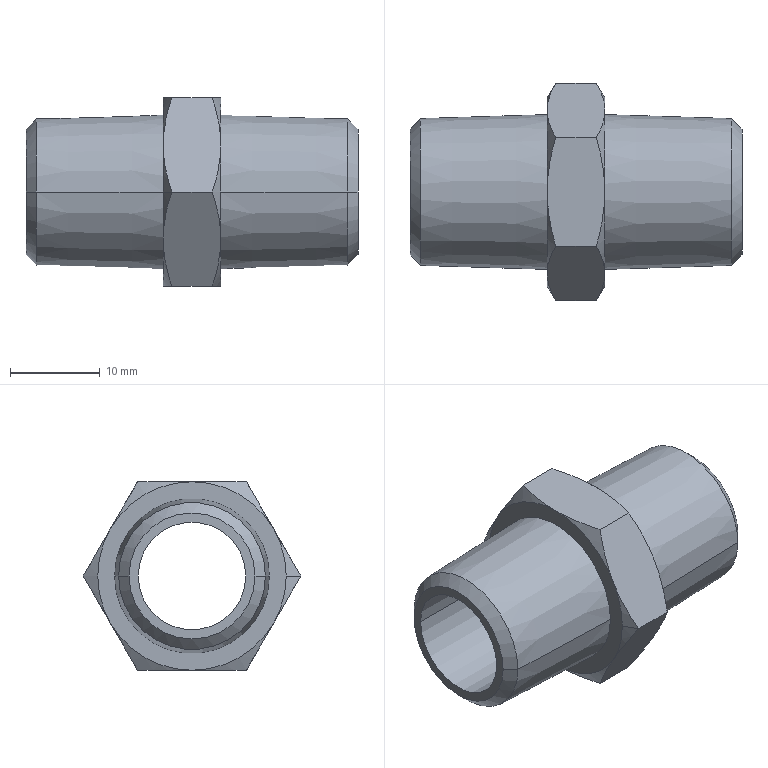Part | NX | 1 solid | 34 faces | box 37 x 24.249 x 21 mm | volume 4927 mm3 | cone 22 | plane 10 | cylinder 2 | commonest cylinder face diameters 12.014 x2
STEP:
#1=CARTESIAN_POINT('',(-17.334,-8.183,0.));
#2=VERTEX_POINT('',#1);
#3=CARTESIAN_POINT('',(-17.334,8.183,0.));
#4=VERTEX_POINT('',#3);
#5=CARTESIAN_POINT('',(-17.334,0.,0.));
#6=DIRECTION('',(-1.,0.,0.));
#7=DIRECTION('',(0.,1.,0.));
#8=AXIS2_PLACEMENT_3D('',#5,#6,#7);
#9=CIRCLE('',#8,8.183);
#10=EDGE_CURVE('',#2,#4,#9,.T.);
#11=ORIENTED_EDGE('',*,*,#10,.T.);
#12=CARTESIAN_POINT('',(-18.5,7.017,0.));
#13=VERTEX_POINT('',#12);
#14=CARTESIAN_POINT('',(-17.917,7.6,0.));
#15=DIRECTION('',(0.7071,0.7071,0.));
#16=VECTOR('',#15,1000.);
#17=LINE('',#14,#16);
#18=EDGE_CURVE('',#4,#13,#17,.F.);
#19=ORIENTED_EDGE('',*,*,#18,.T.);
#20=CARTESIAN_POINT('',(-18.5,-7.017,0.));
#21=VERTEX_POINT('',#20);
#22=CARTESIAN_POINT('',(-18.5,0.,0.));
#23=DIRECTION('',(1.,0.,0.));
#24=DIRECTION('',(0.,1.,0.));
#25=AXIS2_PLACEMENT_3D('',#22,#23,#24);
#26=CIRCLE('',#25,7.017);
#27=EDGE_CURVE('',#13,#21,#26,.T.);
#28=ORIENTED_EDGE('',*,*,#27,.T.);
#29=CARTESIAN_POINT('',(-17.917,-7.6,0.));
#30=DIRECTION('',(0.7071,-0.7071,0.));
#31=VECTOR('',#30,1000.);
#32=LINE('',#29,#31);
#33=EDGE_CURVE('',#2,#21,#32,.F.);
#34=ORIENTED_EDGE('',*,*,#33,.F.);
#35=EDGE_LOOP('',(#11,#19,#28,#34));
#36=FACE_BOUND('',#35,.T.);
#37=CARTESIAN_POINT('',(-17.917,0.,0.));
#38=DIRECTION('',(1.,0.,0.));
#39=DIRECTION('',(0.,-1.,0.));
#40=AXIS2_PLACEMENT_3D('',#37,#38,#39);
#41=CONICAL_SURFACE('',#40,7.6,0.7854);
#42=ADVANCED_FACE('',(#36),#41,.T.);
#43=CARTESIAN_POINT('',(18.5,-6.007,0.));
#44=VERTEX_POINT('',#43);
#45=CARTESIAN_POINT('',(18.5,6.007,0.));
#46=VERTEX_POINT('',#45);
#47=CARTESIAN_POINT('',(18.5,0.,0.));
#48=DIRECTION('',(1.,0.,0.));
#49=DIRECTION('',(0.,1.,0.));
#50=AXIS2_PLACEMENT_3D('',#47,#48,#49);
#51=CIRCLE('',#50,6.007);
#52=EDGE_CURVE('',#44,#46,#51,.T.);
#53=ORIENTED_EDGE('',*,*,#52,.T.);
#54=CARTESIAN_POINT('',(-18.5,6.007,0.));
#55=VERTEX_POINT('',#54);
#56=CARTESIAN_POINT('',(0.,6.007,0.));
#57=DIRECTION('',(1.,0.,0.));
#58=VECTOR('',#57,1000.);
#59=LINE('',#56,#58);
#60=EDGE_CURVE('',#55,#46,#59,.T.);
#61=ORIENTED_EDGE('',*,*,#60,.F.);
#62=CARTESIAN_POINT('',(-18.5,-6.007,0.));
#63=VERTEX_POINT('',#62);
#64=CARTESIAN_POINT('',(-18.5,0.,0.));
#65=DIRECTION('',(-1.,0.,0.));
#66=DIRECTION('',(0.,1.,0.));
#67=AXIS2_PLACEMENT_3D('',#64,#65,#66);
#68=CIRCLE('',#67,6.007);
#69=EDGE_CURVE('',#55,#63,#68,.T.);
#70=ORIENTED_EDGE('',*,*,#69,.T.);
#71=CARTESIAN_POINT('',(0.,-6.007,0.));
#72=DIRECTION('',(1.,0.,0.));
#73=VECTOR('',#72,1000.);
#74=LINE('',#71,#73);
#75=EDGE_CURVE('',#63,#44,#74,.T.);
#76=ORIENTED_EDGE('',*,*,#75,.T.);
#77=EDGE_LOOP('',(#53,#61,#70,#76));
#78=FACE_BOUND('',#77,.T.);
#79=CARTESIAN_POINT('',(0.,0.,0.));
#80=DIRECTION('',(1.,0.,0.));
#81=DIRECTION('',(0.,1.,0.));
#82=AXIS2_PLACEMENT_3D('',#79,#80,#81);
#83=CYLINDRICAL_SURFACE('',#82,6.007);
#84=ADVANCED_FACE('',(#78),#83,.F.);
#85=CARTESIAN_POINT('',(-3.2,-8.625,0.));
#86=VERTEX_POINT('',#85);
#87=CARTESIAN_POINT('',(-3.2,8.625,0.));
#88=VERTEX_POINT('',#87);
#89=CARTESIAN_POINT('',(-3.2,0.,0.));
#90=DIRECTION('',(-1.,0.,0.));
#91=DIRECTION('',(0.,1.,0.));
#92=AXIS2_PLACEMENT_3D('',#89,#90,#91);
#93=CIRCLE('',#92,8.625);
#94=EDGE_CURVE('',#86,#88,#93,.T.);
#95=ORIENTED_EDGE('',*,*,#94,.T.);
#96=CARTESIAN_POINT('',(-10.267,8.404,0.));
#97=DIRECTION('',(0.9995,0.03124,0.));
#98=VECTOR('',#97,1000.);
#99=LINE('',#96,#98);
#100=EDGE_CURVE('',#88,#4,#99,.F.);
#101=ORIENTED_EDGE('',*,*,#100,.T.);
#102=ORIENTED_EDGE('',*,*,#10,.F.);
#103=CARTESIAN_POINT('',(-10.267,-8.404,0.));
#104=DIRECTION('',(0.9995,-0.03124,0.));
#105=VECTOR('',#104,1000.);
#106=LINE('',#103,#105);
#107=EDGE_CURVE('',#86,#2,#106,.F.);
#108=ORIENTED_EDGE('',*,*,#107,.F.);
#109=EDGE_LOOP('',(#95,#101,#102,#108));
#110=FACE_BOUND('',#109,.T.);
#111=CARTESIAN_POINT('',(-10.267,0.,0.));
#112=DIRECTION('',(1.,0.,0.));
#113=DIRECTION('',(0.,-1.,0.));
#114=AXIS2_PLACEMENT_3D('',#111,#112,#113);
#115=CONICAL_SURFACE('',#114,8.404,0.03124);
#116=ADVANCED_FACE('',(#110),#115,.T.);
#117=CARTESIAN_POINT('',(18.5,7.017,0.));
#118=VERTEX_POINT('',#117);
#119=CARTESIAN_POINT('',(18.5,-7.017,0.));
#120=VERTEX_POINT('',#119);
#121=CARTESIAN_POINT('',(18.5,0.,0.));
#122=DIRECTION('',(-1.,0.,0.));
#123=DIRECTION('',(0.,1.,0.));
#124=AXIS2_PLACEMENT_3D('',#121,#122,#123);
#125=CIRCLE('',#124,7.017);
#126=EDGE_CURVE('',#118,#120,#125,.T.);
#127=ORIENTED_EDGE('',*,*,#126,.T.);
#128=CARTESIAN_POINT('',(17.334,-8.183,0.));
#129=VERTEX_POINT('',#128);
#130=CARTESIAN_POINT('',(17.917,-7.6,0.));
#131=DIRECTION('',(-0.7071,-0.7071,0.));
#132=VECTOR('',#131,1000.);
#133=LINE('',#130,#132);
#134=EDGE_CURVE('',#120,#129,#133,.T.);
#135=ORIENTED_EDGE('',*,*,#134,.T.);
#136=CARTESIAN_POINT('',(17.334,8.183,0.));
#137=VERTEX_POINT('',#136);
#138=CARTESIAN_POINT('',(17.334,0.,0.));
#139=DIRECTION('',(-1.,0.,0.));
#140=DIRECTION('',(0.,1.,0.));
#141=AXIS2_PLACEMENT_3D('',#138,#139,#140);
#142=CIRCLE('',#141,8.183);
#143=EDGE_CURVE('',#137,#129,#142,.T.);
#144=ORIENTED_EDGE('',*,*,#143,.F.);
#145=CARTESIAN_POINT('',(17.917,7.6,0.));
#146=DIRECTION('',(-0.7071,0.7071,0.));
#147=VECTOR('',#146,1000.);
#148=LINE('',#145,#147);
#149=EDGE_CURVE('',#118,#137,#148,.T.);
#150=ORIENTED_EDGE('',*,*,#149,.F.);
#151=EDGE_LOOP('',(#127,#135,#144,#150));
#152=FACE_BOUND('',#151,.T.);
#153=CARTESIAN_POINT('',(17.917,0.,0.));
#154=DIRECTION('',(-1.,0.,0.));
#155=DIRECTION('',(0.,1.,0.));
#156=AXIS2_PLACEMENT_3D('',#153,#154,#155);
#157=CONICAL_SURFACE('',#156,7.6,0.7854);
#158=ADVANCED_FACE('',(#152),#157,.T.);
#159=CARTESIAN_POINT('',(-3.2,9.093,-5.25));
#160=VERTEX_POINT('',#159);
#161=CARTESIAN_POINT('',(-3.2,9.093,5.25));
#162=VERTEX_POINT('',#161);
#163=CARTESIAN_POINT('',(-3.2,0.,0.));
#164=DIRECTION('',(1.,0.,0.));
#165=DIRECTION('',(0.,0.866,-0.5));
#166=AXIS2_PLACEMENT_3D('',#163,#164,#165);
#167=CIRCLE('',#166,10.5);
#168=EDGE_CURVE('',#160,#162,#167,.T.);
#169=ORIENTED_EDGE('',*,*,#168,.F.);
#170=CARTESIAN_POINT('',(-3.2,0.,-10.5));
#171=VERTEX_POINT('',#170);
#172=CARTESIAN_POINT('',(-3.2,0.,0.));
#173=DIRECTION('',(1.,0.,0.));
#174=DIRECTION('',(0.,0.,-1.));
#175=AXIS2_PLACEMENT_3D('',#172,#173,#174);
#176=CIRCLE('',#175,10.5);
#177=EDGE_CURVE('',#171,#160,#176,.T.);
#178=ORIENTED_EDGE('',*,*,#177,.F.);
#179=CARTESIAN_POINT('',(-3.2,-9.093,-5.25));
#180=VERTEX_POINT('',#179);
#181=CARTESIAN_POINT('',(-3.2,0.,0.));
#182=DIRECTION('',(1.,0.,0.));
#183=DIRECTION('',(0.,-0.866,-0.5));
#184=AXIS2_PLACEMENT_3D('',#181,#182,#183);
#185=CIRCLE('',#184,10.5);
#186=EDGE_CURVE('',#180,#171,#185,.T.);
#187=ORIENTED_EDGE('',*,*,#186,.F.);
#188=CARTESIAN_POINT('',(-3.2,-10.5,0.));
#189=VERTEX_POINT('',#188);
#190=CARTESIAN_POINT('',(-3.2,0.,0.));
#191=DIRECTION('',(1.,0.,0.));
#192=DIRECTION('',(0.,-1.,0.));
#193=AXIS2_PLACEMENT_3D('',#190,#191,#192);
#194=CIRCLE('',#193,10.5);
#195=EDGE_CURVE('',#189,#180,#194,.T.);
#196=ORIENTED_EDGE('',*,*,#195,.F.);
#197=CARTESIAN_POINT('',(-3.2,-9.093,5.25));
#198=VERTEX_POINT('',#197);
#199=CARTESIAN_POINT('',(-3.2,0.,0.));
#200=DIRECTION('',(1.,0.,0.));
#201=DIRECTION('',(0.,-1.,0.));
#202=AXIS2_PLACEMENT_3D('',#199,#200,#201);
#203=CIRCLE('',#202,10.5);
#204=EDGE_CURVE('',#198,#189,#203,.T.);
#205=ORIENTED_EDGE('',*,*,#204,.F.);
#206=CARTESIAN_POINT('',(-3.2,0.,10.5));
#207=VERTEX_POINT('',#206);
#208=CARTESIAN_POINT('',(-3.2,0.,0.));
#209=DIRECTION('',(1.,0.,0.));
#210=DIRECTION('',(0.,0.,1.));
#211=AXIS2_PLACEMENT_3D('',#208,#209,#210);
#212=CIRCLE('',#211,10.5);
#213=EDGE_CURVE('',#207,#198,#212,.T.);
#214=ORIENTED_EDGE('',*,*,#213,.F.);
#215=CARTESIAN_POINT('',(-3.2,0.,0.));
#216=DIRECTION('',(1.,0.,0.));
#217=DIRECTION('',(0.,0.866,0.5));
#218=AXIS2_PLACEMENT_3D('',#215,#216,#217);
#219=CIRCLE('',#218,10.5);
#220=EDGE_CURVE('',#162,#207,#219,.T.);
#221=ORIENTED_EDGE('',*,*,#220,.F.);
#222=EDGE_LOOP('',(#169,#178,#187,#196,#205,#214,#221));
#223=FACE_BOUND('',#222,.T.);
#224=ORIENTED_EDGE('',*,*,#94,.F.);
#225=CARTESIAN_POINT('',(-3.2,0.,0.));
#226=DIRECTION('',(-1.,0.,0.));
#227=DIRECTION('',(0.,1.,0.));
#228=AXIS2_PLACEMENT_3D('',#225,#226,#227);
#229=CIRCLE('',#228,8.625);
#230=EDGE_CURVE('',#88,#86,#229,.T.);
#231=ORIENTED_EDGE('',*,*,#230,.F.);
#232=EDGE_LOOP('',(#224,#231));
#233=FACE_BOUND('',#232,.T.);
#234=CARTESIAN_POINT('',(-3.2,9.562,0.));
#235=DIRECTION('',(-1.,0.,0.));
#236=DIRECTION('',(0.,0.,1.));
#237=AXIS2_PLACEMENT_3D('',#234,#235,#236);
#238=PLANE('',#237);
#239=ADVANCED_FACE('',(#223,#233),#238,.T.);
#240=ORIENTED_EDGE('',*,*,#168,.T.);
#241=CARTESIAN_POINT('',(-2.262,12.124,0.));
#242=VERTEX_POINT('',#241);
#243=CARTESIAN_POINT('',(-2.262,12.124,0.));
#244=CARTESIAN_POINT('',(-2.577,11.58,0.9435));
#245=CARTESIAN_POINT('',(-3.027,10.608,2.626));
#246=CARTESIAN_POINT('',(-3.2,9.577,4.413));
#247=CARTESIAN_POINT('',(-3.2,9.093,5.25));
#248=B_SPLINE_CURVE_WITH_KNOTS('',3,(#243,#244,#245,#246,#247),.UNSPECIFIED.,.F.,.F.,(4,1,4),(0.,0.5,1.),.UNSPECIFIED.);
#249=EDGE_CURVE('',#242,#162,#248,.T.);
#250=ORIENTED_EDGE('',*,*,#249,.F.);
#251=CARTESIAN_POINT('',(-3.2,9.093,-5.25));
#252=CARTESIAN_POINT('',(-3.2,9.58,-4.407));
#253=CARTESIAN_POINT('',(-3.032,10.59,-2.657));
#254=CARTESIAN_POINT('',(-2.575,11.583,-0.9375));
#255=CARTESIAN_POINT('',(-2.262,12.124,0.));
#256=B_SPLINE_CURVE_WITH_KNOTS('',3,(#251,#252,#253,#254,#255),.UNSPECIFIED.,.F.,.F.,(4,1,4),(0.,0.5,1.),.UNSPECIFIED.);
#257=EDGE_CURVE('',#160,#242,#256,.T.);
#258=ORIENTED_EDGE('',*,*,#257,.F.);
#259=EDGE_LOOP('',(#240,#250,#258));
#260=FACE_BOUND('',#259,.T.);
#261=CARTESIAN_POINT('',(-2.731,0.,0.));
#262=DIRECTION('',(1.,0.,0.));
#263=DIRECTION('',(0.,-1.,0.));
#264=AXIS2_PLACEMENT_3D('',#261,#262,#263);
#265=CONICAL_SURFACE('',#264,11.312,1.047);
#266=ADVANCED_FACE('',(#260),#265,.T.);
#267=CARTESIAN_POINT('',(3.2,8.625,0.));
#268=VERTEX_POINT('',#267);
#269=CARTESIAN_POINT('',(3.2,-8.625,0.));
#270=VERTEX_POINT('',#269);
#271=CARTESIAN_POINT('',(3.2,0.,0.));
#272=DIRECTION('',(1.,0.,0.));
#273=DIRECTION('',(0.,1.,0.));
#274=AXIS2_PLACEMENT_3D('',#271,#272,#273);
#275=CIRCLE('',#274,8.625);
#276=EDGE_CURVE('',#268,#270,#275,.T.);
#277=ORIENTED_EDGE('',*,*,#276,.T.);
#278=CARTESIAN_POINT('',(10.267,-8.404,0.));
#279=DIRECTION('',(-0.9995,-0.03124,0.));
#280=VECTOR('',#279,1000.);
#281=LINE('',#278,#280);
#282=EDGE_CURVE('',#270,#129,#281,.F.);
#283=ORIENTED_EDGE('',*,*,#282,.T.);
#284=CARTESIAN_POINT('',(17.334,0.,0.));
#285=DIRECTION('',(-1.,0.,0.));
#286=DIRECTION('',(0.,1.,0.));
#287=AXIS2_PLACEMENT_3D('',#284,#285,#286);
#288=CIRCLE('',#287,8.183);
#289=EDGE_CURVE('',#129,#137,#288,.T.);
#290=ORIENTED_EDGE('',*,*,#289,.T.);
#291=CARTESIAN_POINT('',(10.267,8.404,0.));
#292=DIRECTION('',(-0.9995,0.03124,0.));
#293=VECTOR('',#292,1000.);
#294=LINE('',#291,#293);
#295=EDGE_CURVE('',#268,#137,#294,.F.);
#296=ORIENTED_EDGE('',*,*,#295,.F.);
#297=EDGE_LOOP('',(#277,#283,#290,#296));
#298=FACE_BOUND('',#297,.T.);
#299=CARTESIAN_POINT('',(10.267,0.,0.));
#300=DIRECTION('',(-1.,0.,0.));
#301=DIRECTION('',(0.,1.,0.));
#302=AXIS2_PLACEMENT_3D('',#299,#300,#301);
#303=CONICAL_SURFACE('',#302,8.404,0.03124);
#304=ADVANCED_FACE('',(#298),#303,.T.);
#305=CARTESIAN_POINT('',(-2.262,6.062,-10.5));
#306=VERTEX_POINT('',#305);
#307=CARTESIAN_POINT('',(-2.262,6.062,-10.5));
#308=CARTESIAN_POINT('',(-2.577,6.607,-9.556));
#309=CARTESIAN_POINT('',(-3.027,7.578,-7.874));
#310=CARTESIAN_POINT('',(-3.2,8.61,-6.087));
#311=CARTESIAN_POINT('',(-3.2,9.093,-5.25));
#312=B_SPLINE_CURVE_WITH_KNOTS('',3,(#307,#308,#309,#310,#311),.UNSPECIFIED.,.F.,.F.,(4,1,4),(0.,0.5,1.),.UNSPECIFIED.);
#313=EDGE_CURVE('',#306,#160,#312,.T.);
#314=ORIENTED_EDGE('',*,*,#313,.T.);
#315=ORIENTED_EDGE('',*,*,#257,.T.);
#316=CARTESIAN_POINT('',(2.262,12.124,0.));
#317=VERTEX_POINT('',#316);
#318=CARTESIAN_POINT('',(2.262,12.124,0.));
#319=DIRECTION('',(-1.,0.,0.));
#320=VECTOR('',#319,1000.);
#321=LINE('',#318,#320);
#322=EDGE_CURVE('',#317,#242,#321,.T.);
#323=ORIENTED_EDGE('',*,*,#322,.F.);
#324=CARTESIAN_POINT('',(3.2,9.093,-5.25));
#325=VERTEX_POINT('',#324);
#326=CARTESIAN_POINT('',(2.262,12.124,0.));
#327=CARTESIAN_POINT('',(2.577,11.58,-0.9435));
#328=CARTESIAN_POINT('',(3.027,10.608,-2.626));
#329=CARTESIAN_POINT('',(3.2,9.577,-4.413));
#330=CARTESIAN_POINT('',(3.2,9.093,-5.25));
#331=B_SPLINE_CURVE_WITH_KNOTS('',3,(#326,#327,#328,#329,#330),.UNSPECIFIED.,.F.,.F.,(4,1,4),(0.,0.5,1.),.UNSPECIFIED.);
#332=EDGE_CURVE('',#317,#325,#331,.T.);
#333=ORIENTED_EDGE('',*,*,#332,.T.);
#334=CARTESIAN_POINT('',(2.262,6.062,-10.5));
#335=VERTEX_POINT('',#334);
#336=CARTESIAN_POINT('',(3.2,9.093,-5.25));
#337=CARTESIAN_POINT('',(3.2,8.606,-6.093));
#338=CARTESIAN_POINT('',(3.032,7.596,-7.843));
#339=CARTESIAN_POINT('',(2.575,6.603,-9.563));
#340=CARTESIAN_POINT('',(2.262,6.062,-10.5));
#341=B_SPLINE_CURVE_WITH_KNOTS('',3,(#336,#337,#338,#339,#340),.UNSPECIFIED.,.F.,.F.,(4,1,4),(0.,0.5,1.),.UNSPECIFIED.);
#342=EDGE_CURVE('',#325,#335,#341,.T.);
#343=ORIENTED_EDGE('',*,*,#342,.T.);
#344=CARTESIAN_POINT('',(2.262,6.062,-10.5));
#345=DIRECTION('',(-1.,0.,0.));
#346=VECTOR('',#345,1000.);
#347=LINE('',#344,#346);
#348=EDGE_CURVE('',#335,#306,#347,.T.);
#349=ORIENTED_EDGE('',*,*,#348,.T.);
#350=EDGE_LOOP('',(#314,#315,#323,#333,#343,#349));
#351=FACE_BOUND('',#350,.T.);
#352=CARTESIAN_POINT('',(4.,12.124,0.));
#353=DIRECTION('',(0.,-0.866,0.5));
#354=DIRECTION('',(-1.,0.,0.));
#355=AXIS2_PLACEMENT_3D('',#352,#353,#354);
#356=PLANE('',#355);
#357=ADVANCED_FACE('',(#351),#356,.F.);
#358=CARTESIAN_POINT('',(-3.2,0.,-10.5));
#359=CARTESIAN_POINT('',(-3.2,0.9737,-10.5));
#360=CARTESIAN_POINT('',(-3.032,2.994,-10.5));
#361=CARTESIAN_POINT('',(-2.575,4.98,-10.5));
#362=CARTESIAN_POINT('',(-2.262,6.062,-10.5));
#363=B_SPLINE_CURVE_WITH_KNOTS('',3,(#358,#359,#360,#361,#362),.UNSPECIFIED.,.F.,.F.,(4,1,4),(0.,0.5,1.),.UNSPECIFIED.);
#364=EDGE_CURVE('',#171,#306,#363,.T.);
#365=ORIENTED_EDGE('',*,*,#364,.F.);
#366=ORIENTED_EDGE('',*,*,#177,.T.);
#367=ORIENTED_EDGE('',*,*,#313,.F.);
#368=EDGE_LOOP('',(#365,#366,#367));
#369=FACE_BOUND('',#368,.T.);
#370=CARTESIAN_POINT('',(-2.731,0.,0.));
#371=DIRECTION('',(1.,0.,0.));
#372=DIRECTION('',(0.,-1.,0.));
#373=AXIS2_PLACEMENT_3D('',#370,#371,#372);
#374=CONICAL_SURFACE('',#373,11.312,1.047);
#375=ADVANCED_FACE('',(#369),#374,.T.);
#376=CARTESIAN_POINT('',(-2.262,-6.062,-10.5));
#377=VERTEX_POINT('',#376);
#378=CARTESIAN_POINT('',(-2.262,-6.062,-10.5));
#379=CARTESIAN_POINT('',(-2.577,-4.973,-10.5));
#380=CARTESIAN_POINT('',(-3.027,-3.03,-10.5));
#381=CARTESIAN_POINT('',(-3.2,-0.9668,-10.5));
#382=CARTESIAN_POINT('',(-3.2,0.,-10.5));
#383=B_SPLINE_CURVE_WITH_KNOTS('',3,(#378,#379,#380,#381,#382),.UNSPECIFIED.,.F.,.F.,(4,1,4),(0.,0.5,1.),.UNSPECIFIED.);
#384=EDGE_CURVE('',#377,#171,#383,.T.);
#385=ORIENTED_EDGE('',*,*,#384,.T.);
#386=ORIENTED_EDGE('',*,*,#364,.T.);
#387=ORIENTED_EDGE('',*,*,#348,.F.);
#388=CARTESIAN_POINT('',(3.2,0.,-10.5));
#389=VERTEX_POINT('',#388);
#390=CARTESIAN_POINT('',(2.262,6.062,-10.5));
#391=CARTESIAN_POINT('',(2.577,4.973,-10.5));
#392=CARTESIAN_POINT('',(3.027,3.03,-10.5));
#393=CARTESIAN_POINT('',(3.2,0.9668,-10.5));
#394=CARTESIAN_POINT('',(3.2,0.,-10.5));
#395=B_SPLINE_CURVE_WITH_KNOTS('',3,(#390,#391,#392,#393,#394),.UNSPECIFIED.,.F.,.F.,(4,1,4),(0.,0.5,1.),.UNSPECIFIED.);
#396=EDGE_CURVE('',#335,#389,#395,.T.);
#397=ORIENTED_EDGE('',*,*,#396,.T.);
#398=CARTESIAN_POINT('',(2.262,-6.062,-10.5));
#399=VERTEX_POINT('',#398);
#400=CARTESIAN_POINT('',(3.2,0.,-10.5));
#401=CARTESIAN_POINT('',(3.2,-0.9737,-10.5));
#402=CARTESIAN_POINT('',(3.032,-2.994,-10.5));
#403=CARTESIAN_POINT('',(2.575,-4.98,-10.5));
#404=CARTESIAN_POINT('',(2.262,-6.062,-10.5));
#405=B_SPLINE_CURVE_WITH_KNOTS('',3,(#400,#401,#402,#403,#404),.UNSPECIFIED.,.F.,.F.,(4,1,4),(0.,0.5,1.),.UNSPECIFIED.);
#406=EDGE_CURVE('',#389,#399,#405,.T.);
#407=ORIENTED_EDGE('',*,*,#406,.T.);
#408=CARTESIAN_POINT('',(2.262,-6.062,-10.5));
#409=DIRECTION('',(-1.,0.,0.));
#410=VECTOR('',#409,1000.);
#411=LINE('',#408,#410);
#412=EDGE_CURVE('',#399,#377,#411,.T.);
#413=ORIENTED_EDGE('',*,*,#412,.T.);
#414=EDGE_LOOP('',(#385,#386,#387,#397,#407,#413));
#415=FACE_BOUND('',#414,.T.);
#416=CARTESIAN_POINT('',(4.,6.062,-10.5));
#417=DIRECTION('',(0.,0.,1.));
#418=DIRECTION('',(1.,0.,0.));
#419=AXIS2_PLACEMENT_3D('',#416,#417,#418);
#420=PLANE('',#419);
#421=ADVANCED_FACE('',(#415),#420,.F.);
#422=CARTESIAN_POINT('',(-3.2,-9.093,-5.25));
#423=CARTESIAN_POINT('',(-3.2,-8.606,-6.093));
#424=CARTESIAN_POINT('',(-3.032,-7.596,-7.843));
#425=CARTESIAN_POINT('',(-2.575,-6.603,-9.563));
#426=CARTESIAN_POINT('',(-2.262,-6.062,-10.5));
#427=B_SPLINE_CURVE_WITH_KNOTS('',3,(#422,#423,#424,#425,#426),.UNSPECIFIED.,.F.,.F.,(4,1,4),(0.,0.5,1.),.UNSPECIFIED.);
#428=EDGE_CURVE('',#180,#377,#427,.T.);
#429=ORIENTED_EDGE('',*,*,#428,.F.);
#430=ORIENTED_EDGE('',*,*,#186,.T.);
#431=ORIENTED_EDGE('',*,*,#384,.F.);
#432=EDGE_LOOP('',(#429,#430,#431));
#433=FACE_BOUND('',#432,.T.);
#434=CARTESIAN_POINT('',(-2.731,0.,0.));
#435=DIRECTION('',(1.,0.,0.));
#436=DIRECTION('',(0.,-1.,0.));
#437=AXIS2_PLACEMENT_3D('',#434,#435,#436);
#438=CONICAL_SURFACE('',#437,11.312,1.047);
#439=ADVANCED_FACE('',(#433),#438,.T.);
#440=CARTESIAN_POINT('',(-2.262,-12.124,0.));
#441=VERTEX_POINT('',#440);
#442=CARTESIAN_POINT('',(-2.262,-12.124,0.));
#443=CARTESIAN_POINT('',(-2.577,-11.58,-0.9435));
#444=CARTESIAN_POINT('',(-3.027,-10.608,-2.626));
#445=CARTESIAN_POINT('',(-3.2,-9.577,-4.413));
#446=CARTESIAN_POINT('',(-3.2,-9.093,-5.25));
#447=B_SPLINE_CURVE_WITH_KNOTS('',3,(#442,#443,#444,#445,#446),.UNSPECIFIED.,.F.,.F.,(4,1,4),(0.,0.5,1.),.UNSPECIFIED.);
#448=EDGE_CURVE('',#441,#180,#447,.T.);
#449=ORIENTED_EDGE('',*,*,#448,.T.);
#450=ORIENTED_EDGE('',*,*,#428,.T.);
#451=ORIENTED_EDGE('',*,*,#412,.F.);
#452=CARTESIAN_POINT('',(3.2,-9.093,-5.25));
#453=VERTEX_POINT('',#452);
#454=CARTESIAN_POINT('',(2.262,-6.062,-10.5));
#455=CARTESIAN_POINT('',(2.577,-6.607,-9.556));
#456=CARTESIAN_POINT('',(3.027,-7.578,-7.874));
#457=CARTESIAN_POINT('',(3.2,-8.61,-6.087));
#458=CARTESIAN_POINT('',(3.2,-9.093,-5.25));
#459=B_SPLINE_CURVE_WITH_KNOTS('',3,(#454,#455,#456,#457,#458),.UNSPECIFIED.,.F.,.F.,(4,1,4),(0.,0.5,1.),.UNSPECIFIED.);
#460=EDGE_CURVE('',#399,#453,#459,.T.);
#461=ORIENTED_EDGE('',*,*,#460,.T.);
#462=CARTESIAN_POINT('',(2.262,-12.124,0.));
#463=VERTEX_POINT('',#462);
#464=CARTESIAN_POINT('',(3.2,-9.093,-5.25));
#465=CARTESIAN_POINT('',(3.2,-9.58,-4.407));
#466=CARTESIAN_POINT('',(3.032,-10.59,-2.657));
#467=CARTESIAN_POINT('',(2.575,-11.583,-0.9375));
#468=CARTESIAN_POINT('',(2.262,-12.124,0.));
#469=B_SPLINE_CURVE_WITH_KNOTS('',3,(#464,#465,#466,#467,#468),.UNSPECIFIED.,.F.,.F.,(4,1,4),(0.,0.5,1.),.UNSPECIFIED.);
#470=EDGE_CURVE('',#453,#463,#469,.T.);
#471=ORIENTED_EDGE('',*,*,#470,.T.);
#472=CARTESIAN_POINT('',(2.262,-12.124,0.));
#473=DIRECTION('',(-1.,0.,0.));
#474=VECTOR('',#473,1000.);
#475=LINE('',#472,#474);
#476=EDGE_CURVE('',#463,#441,#475,.T.);
#477=ORIENTED_EDGE('',*,*,#476,.T.);
#478=EDGE_LOOP('',(#449,#450,#451,#461,#471,#477));
#479=FACE_BOUND('',#478,.T.);
#480=CARTESIAN_POINT('',(4.,-6.062,-10.5));
#481=DIRECTION('',(0.,0.866,0.5));
#482=DIRECTION('',(1.,0.,0.));
#483=AXIS2_PLACEMENT_3D('',#480,#481,#482);
#484=PLANE('',#483);
#485=ADVANCED_FACE('',(#479),#484,.F.);
#486=CARTESIAN_POINT('',(-2.731,-11.312,0.));
#487=DIRECTION('',(0.5,-0.866,0.));
#488=VECTOR('',#487,1000.);
#489=LINE('',#486,#488);
#490=EDGE_CURVE('',#189,#441,#489,.T.);
#491=ORIENTED_EDGE('',*,*,#490,.F.);
#492=ORIENTED_EDGE('',*,*,#195,.T.);
#493=ORIENTED_EDGE('',*,*,#448,.F.);
#494=EDGE_LOOP('',(#491,#492,#493));
#495=FACE_BOUND('',#494,.T.);
#496=CARTESIAN_POINT('',(-2.731,0.,0.));
#497=DIRECTION('',(1.,0.,0.));
#498=DIRECTION('',(0.,-1.,0.));
#499=AXIS2_PLACEMENT_3D('',#496,#497,#498);
#500=CONICAL_SURFACE('',#499,11.312,1.047);
#501=ADVANCED_FACE('',(#495),#500,.T.);
#502=CARTESIAN_POINT('',(2.262,6.062,10.5));
#503=VERTEX_POINT('',#502);
#504=CARTESIAN_POINT('',(3.2,9.093,5.25));
#505=VERTEX_POINT('',#504);
#506=CARTESIAN_POINT('',(2.262,6.062,10.5));
#507=CARTESIAN_POINT('',(2.577,6.607,9.556));
#508=CARTESIAN_POINT('',(3.027,7.578,7.874));
#509=CARTESIAN_POINT('',(3.2,8.61,6.087));
#510=CARTESIAN_POINT('',(3.2,9.093,5.25));
#511=B_SPLINE_CURVE_WITH_KNOTS('',3,(#506,#507,#508,#509,#510),.UNSPECIFIED.,.F.,.F.,(4,1,4),(0.,0.5,1.),.UNSPECIFIED.);
#512=EDGE_CURVE('',#503,#505,#511,.T.);
#513=ORIENTED_EDGE('',*,*,#512,.F.);
#514=CARTESIAN_POINT('',(3.2,0.,10.5));
#515=VERTEX_POINT('',#514);
#516=CARTESIAN_POINT('',(3.2,0.,10.5));
#517=CARTESIAN_POINT('',(3.2,0.9737,10.5));
#518=CARTESIAN_POINT('',(3.032,2.994,10.5));
#519=CARTESIAN_POINT('',(2.575,4.98,10.5));
#520=CARTESIAN_POINT('',(2.262,6.062,10.5));
#521=B_SPLINE_CURVE_WITH_KNOTS('',3,(#516,#517,#518,#519,#520),.UNSPECIFIED.,.F.,.F.,(4,1,4),(0.,0.5,1.),.UNSPECIFIED.);
#522=EDGE_CURVE('',#515,#503,#521,.T.);
#523=ORIENTED_EDGE('',*,*,#522,.F.);
#524=CARTESIAN_POINT('',(3.2,0.,0.));
#525=DIRECTION('',(-1.,0.,0.));
#526=DIRECTION('',(0.,0.,1.));
#527=AXIS2_PLACEMENT_3D('',#524,#525,#526);
#528=CIRCLE('',#527,10.5);
#529=EDGE_CURVE('',#515,#505,#528,.T.);
#530=ORIENTED_EDGE('',*,*,#529,.T.);
#531=EDGE_LOOP('',(#513,#523,#530));
#532=FACE_BOUND('',#531,.T.);
#533=CARTESIAN_POINT('',(2.731,0.,0.));
#534=DIRECTION('',(-1.,0.,0.));
#535=DIRECTION('',(0.,1.,0.));
#536=AXIS2_PLACEMENT_3D('',#533,#534,#535);
#537=CONICAL_SURFACE('',#536,11.312,1.047);
#538=ADVANCED_FACE('',(#532),#537,.T.);
#539=CARTESIAN_POINT('',(-3.2,-9.093,5.25));
#540=CARTESIAN_POINT('',(-3.2,-9.58,4.407));
#541=CARTESIAN_POINT('',(-3.032,-10.59,2.657));
#542=CARTESIAN_POINT('',(-2.575,-11.583,0.9375));
#543=CARTESIAN_POINT('',(-2.262,-12.124,0.));
#544=B_SPLINE_CURVE_WITH_KNOTS('',3,(#539,#540,#541,#542,#543),.UNSPECIFIED.,.F.,.F.,(4,1,4),(0.,0.5,1.),.UNSPECIFIED.);
#545=EDGE_CURVE('',#198,#441,#544,.T.);
#546=ORIENTED_EDGE('',*,*,#545,.T.);
#547=ORIENTED_EDGE('',*,*,#476,.F.);
#548=CARTESIAN_POINT('',(3.2,-9.093,5.25));
#549=VERTEX_POINT('',#548);
#550=CARTESIAN_POINT('',(2.262,-12.124,0.));
#551=CARTESIAN_POINT('',(2.577,-11.58,0.9435));
#552=CARTESIAN_POINT('',(3.027,-10.608,2.626));
#553=CARTESIAN_POINT('',(3.2,-9.577,4.413));
#554=CARTESIAN_POINT('',(3.2,-9.093,5.25));
#555=B_SPLINE_CURVE_WITH_KNOTS('',3,(#550,#551,#552,#553,#554),.UNSPECIFIED.,.F.,.F.,(4,1,4),(0.,0.5,1.),.UNSPECIFIED.);
#556=EDGE_CURVE('',#463,#549,#555,.T.);
#557=ORIENTED_EDGE('',*,*,#556,.T.);
#558=CARTESIAN_POINT('',(2.262,-6.062,10.5));
#559=VERTEX_POINT('',#558);
#560=CARTESIAN_POINT('',(3.2,-9.093,5.25));
#561=CARTESIAN_POINT('',(3.2,-8.606,6.093));
#562=CARTESIAN_POINT('',(3.032,-7.596,7.843));
#563=CARTESIAN_POINT('',(2.575,-6.603,9.563));
#564=CARTESIAN_POINT('',(2.262,-6.062,10.5));
#565=B_SPLINE_CURVE_WITH_KNOTS('',3,(#560,#561,#562,#563,#564),.UNSPECIFIED.,.F.,.F.,(4,1,4),(0.,0.5,1.),.UNSPECIFIED.);
#566=EDGE_CURVE('',#549,#559,#565,.T.);
#567=ORIENTED_EDGE('',*,*,#566,.T.);
#568=CARTESIAN_POINT('',(-2.262,-6.062,10.5));
#569=VERTEX_POINT('',#568);
#570=CARTESIAN_POINT('',(2.262,-6.062,10.5));
#571=DIRECTION('',(-1.,0.,0.));
#572=VECTOR('',#571,1000.);
#573=LINE('',#570,#572);
#574=EDGE_CURVE('',#559,#569,#573,.T.);
#575=ORIENTED_EDGE('',*,*,#574,.T.);
#576=CARTESIAN_POINT('',(-2.262,-6.062,10.5));
#577=CARTESIAN_POINT('',(-2.577,-6.607,9.556));
#578=CARTESIAN_POINT('',(-3.027,-7.578,7.874));
#579=CARTESIAN_POINT('',(-3.2,-8.61,6.087));
#580=CARTESIAN_POINT('',(-3.2,-9.093,5.25));
#581=B_SPLINE_CURVE_WITH_KNOTS('',3,(#576,#577,#578,#579,#580),.UNSPECIFIED.,.F.,.F.,(4,1,4),(0.,0.5,1.),.UNSPECIFIED.);
#582=EDGE_CURVE('',#569,#198,#581,.T.);
#583=ORIENTED_EDGE('',*,*,#582,.T.);
#584=EDGE_LOOP('',(#546,#547,#557,#567,#575,#583));
#585=FACE_BOUND('',#584,.T.);
#586=CARTESIAN_POINT('',(4.,-12.124,0.));
#587=DIRECTION('',(0.,0.866,-0.5));
#588=DIRECTION('',(-1.,0.,0.));
#589=AXIS2_PLACEMENT_3D('',#586,#587,#588);
#590=PLANE('',#589);
#591=ADVANCED_FACE('',(#585),#590,.F.);
#592=ORIENTED_EDGE('',*,*,#582,.F.);
#593=CARTESIAN_POINT('',(-3.2,0.,10.5));
#594=CARTESIAN_POINT('',(-3.2,-0.9737,10.5));
#595=CARTESIAN_POINT('',(-3.032,-2.994,10.5));
#596=CARTESIAN_POINT('',(-2.575,-4.98,10.5));
#597=CARTESIAN_POINT('',(-2.262,-6.062,10.5));
#598=B_SPLINE_CURVE_WITH_KNOTS('',3,(#593,#594,#595,#596,#597),.UNSPECIFIED.,.F.,.F.,(4,1,4),(0.,0.5,1.),.UNSPECIFIED.);
#599=EDGE_CURVE('',#207,#569,#598,.T.);
#600=ORIENTED_EDGE('',*,*,#599,.F.);
#601=ORIENTED_EDGE('',*,*,#213,.T.);
#602=EDGE_LOOP('',(#592,#600,#601));
#603=FACE_BOUND('',#602,.T.);
#604=CARTESIAN_POINT('',(-2.731,0.,0.));
#605=DIRECTION('',(1.,0.,0.));
#606=DIRECTION('',(0.,-1.,0.));
#607=AXIS2_PLACEMENT_3D('',#604,#605,#606);
#608=CONICAL_SURFACE('',#607,11.312,1.047);
#609=ADVANCED_FACE('',(#603),#608,.T.);
#610=ORIENTED_EDGE('',*,*,#599,.T.);
#611=ORIENTED_EDGE('',*,*,#574,.F.);
#612=CARTESIAN_POINT('',(2.262,-6.062,10.5));
#613=CARTESIAN_POINT('',(2.577,-4.973,10.5));
#614=CARTESIAN_POINT('',(3.027,-3.03,10.5));
#615=CARTESIAN_POINT('',(3.2,-0.9668,10.5));
#616=CARTESIAN_POINT('',(3.2,0.,10.5));
#617=B_SPLINE_CURVE_WITH_KNOTS('',3,(#612,#613,#614,#615,#616),.UNSPECIFIED.,.F.,.F.,(4,1,4),(0.,0.5,1.),.UNSPECIFIED.);
#618=EDGE_CURVE('',#559,#515,#617,.T.);
#619=ORIENTED_EDGE('',*,*,#618,.T.);
#620=ORIENTED_EDGE('',*,*,#522,.T.);
#621=CARTESIAN_POINT('',(-2.262,6.062,10.5));
#622=VERTEX_POINT('',#621);
#623=CARTESIAN_POINT('',(2.262,6.062,10.5));
#624=DIRECTION('',(-1.,0.,0.));
#625=VECTOR('',#624,1000.);
#626=LINE('',#623,#625);
#627=EDGE_CURVE('',#503,#622,#626,.T.);
#628=ORIENTED_EDGE('',*,*,#627,.T.);
#629=CARTESIAN_POINT('',(-2.262,6.062,10.5));
#630=CARTESIAN_POINT('',(-2.577,4.973,10.5));
#631=CARTESIAN_POINT('',(-3.027,3.03,10.5));
#632=CARTESIAN_POINT('',(-3.2,0.9668,10.5));
#633=CARTESIAN_POINT('',(-3.2,0.,10.5));
#634=B_SPLINE_CURVE_WITH_KNOTS('',3,(#629,#630,#631,#632,#633),.UNSPECIFIED.,.F.,.F.,(4,1,4),(0.,0.5,1.),.UNSPECIFIED.);
#635=EDGE_CURVE('',#622,#207,#634,.T.);
#636=ORIENTED_EDGE('',*,*,#635,.T.);
#637=EDGE_LOOP('',(#610,#611,#619,#620,#628,#636));
#638=FACE_BOUND('',#637,.T.);
#639=CARTESIAN_POINT('',(4.,-6.062,10.5));
#640=DIRECTION('',(0.,0.,-1.));
#641=DIRECTION('',(0.,-1.,0.));
#642=AXIS2_PLACEMENT_3D('',#639,#640,#641);
#643=PLANE('',#642);
#644=ADVANCED_FACE('',(#638),#643,.F.);
#645=ORIENTED_EDGE('',*,*,#635,.F.);
#646=CARTESIAN_POINT('',(-3.2,9.093,5.25));
#647=CARTESIAN_POINT('',(-3.2,8.606,6.093));
#648=CARTESIAN_POINT('',(-3.032,7.596,7.843));
#649=CARTESIAN_POINT('',(-2.575,6.603,9.563));
#650=CARTESIAN_POINT('',(-2.262,6.062,10.5));
#651=B_SPLINE_CURVE_WITH_KNOTS('',3,(#646,#647,#648,#649,#650),.UNSPECIFIED.,.F.,.F.,(4,1,4),(0.,0.5,1.),.UNSPECIFIED.);
#652=EDGE_CURVE('',#162,#622,#651,.T.);
#653=ORIENTED_EDGE('',*,*,#652,.F.);
#654=ORIENTED_EDGE('',*,*,#220,.T.);
#655=EDGE_LOOP('',(#645,#653,#654));
#656=FACE_BOUND('',#655,.T.);
#657=CARTESIAN_POINT('',(-2.731,0.,0.));
#658=DIRECTION('',(1.,0.,0.));
#659=DIRECTION('',(0.,-1.,0.));
#660=AXIS2_PLACEMENT_3D('',#657,#658,#659);
#661=CONICAL_SURFACE('',#660,11.312,1.047);
#662=ADVANCED_FACE('',(#656),#661,.T.);
#663=ORIENTED_EDGE('',*,*,#652,.T.);
#664=ORIENTED_EDGE('',*,*,#627,.F.);
#665=ORIENTED_EDGE('',*,*,#512,.T.);
#666=CARTESIAN_POINT('',(3.2,9.093,5.25));
#667=CARTESIAN_POINT('',(3.2,9.58,4.407));
#668=CARTESIAN_POINT('',(3.032,10.59,2.657));
#669=CARTESIAN_POINT('',(2.575,11.583,0.9375));
#670=CARTESIAN_POINT('',(2.262,12.124,0.));
#671=B_SPLINE_CURVE_WITH_KNOTS('',3,(#666,#667,#668,#669,#670),.UNSPECIFIED.,.F.,.F.,(4,1,4),(0.,0.5,1.),.UNSPECIFIED.);
#672=EDGE_CURVE('',#505,#317,#671,.T.);
#673=ORIENTED_EDGE('',*,*,#672,.T.);
#674=ORIENTED_EDGE('',*,*,#322,.T.);
#675=ORIENTED_EDGE('',*,*,#249,.T.);
#676=EDGE_LOOP('',(#663,#664,#665,#673,#674,#675));
#677=FACE_BOUND('',#676,.T.);
#678=CARTESIAN_POINT('',(4.,6.062,10.5));
#679=DIRECTION('',(0.,-0.866,-0.5));
#680=DIRECTION('',(0.,0.5,-0.866));
#681=AXIS2_PLACEMENT_3D('',#678,#679,#680);
#682=PLANE('',#681);
#683=ADVANCED_FACE('',(#677),#682,.F.);
#684=CARTESIAN_POINT('',(3.2,10.5,0.));
#685=VERTEX_POINT('',#684);
#686=CARTESIAN_POINT('',(2.731,11.312,0.));
#687=DIRECTION('',(-0.5,0.866,0.));
#688=VECTOR('',#687,1000.);
#689=LINE('',#686,#688);
#690=EDGE_CURVE('',#685,#317,#689,.T.);
#691=ORIENTED_EDGE('',*,*,#690,.F.);
#692=CARTESIAN_POINT('',(3.2,0.,0.));
#693=DIRECTION('',(-1.,0.,0.));
#694=DIRECTION('',(0.,0.866,0.5));
#695=AXIS2_PLACEMENT_3D('',#692,#693,#694);
#696=CIRCLE('',#695,10.5);
#697=EDGE_CURVE('',#685,#325,#696,.T.);
#698=ORIENTED_EDGE('',*,*,#697,.T.);
#699=ORIENTED_EDGE('',*,*,#332,.F.);
#700=EDGE_LOOP('',(#691,#698,#699));
#701=FACE_BOUND('',#700,.T.);
#702=CARTESIAN_POINT('',(2.731,0.,0.));
#703=DIRECTION('',(-1.,0.,0.));
#704=DIRECTION('',(0.,1.,0.));
#705=AXIS2_PLACEMENT_3D('',#702,#703,#704);
#706=CONICAL_SURFACE('',#705,11.312,1.047);
#707=ADVANCED_FACE('',(#701),#706,.T.);
#708=ORIENTED_EDGE('',*,*,#126,.F.);
#709=CARTESIAN_POINT('',(18.5,0.,0.));
#710=DIRECTION('',(-1.,0.,0.));
#711=DIRECTION('',(0.,1.,0.));
#712=AXIS2_PLACEMENT_3D('',#709,#710,#711);
#713=CIRCLE('',#712,7.017);
#714=EDGE_CURVE('',#120,#118,#713,.T.);
#715=ORIENTED_EDGE('',*,*,#714,.F.);
#716=EDGE_LOOP('',(#708,#715));
#717=FACE_BOUND('',#716,.T.);
#718=ORIENTED_EDGE('',*,*,#52,.F.);
#719=CARTESIAN_POINT('',(18.5,0.,0.));
#720=DIRECTION('',(1.,0.,0.));
#721=DIRECTION('',(0.,1.,0.));
#722=AXIS2_PLACEMENT_3D('',#719,#720,#721);
#723=CIRCLE('',#722,6.007);
#724=EDGE_CURVE('',#46,#44,#723,.T.);
#725=ORIENTED_EDGE('',*,*,#724,.F.);
#726=EDGE_LOOP('',(#718,#725));
#727=FACE_BOUND('',#726,.T.);
#728=CARTESIAN_POINT('',(18.5,6.512,0.));
#729=DIRECTION('',(1.,0.,0.));
#730=DIRECTION('',(0.,1.,0.));
#731=AXIS2_PLACEMENT_3D('',#728,#729,#730);
#732=PLANE('',#731);
#733=ADVANCED_FACE('',(#717,#727),#732,.T.);
#734=CARTESIAN_POINT('',(3.2,0.,0.));
#735=DIRECTION('',(-1.,0.,0.));
#736=DIRECTION('',(0.,0.866,0.5));
#737=AXIS2_PLACEMENT_3D('',#734,#735,#736);
#738=CIRCLE('',#737,10.5);
#739=EDGE_CURVE('',#505,#685,#738,.T.);
#740=ORIENTED_EDGE('',*,*,#739,.F.);
#741=ORIENTED_EDGE('',*,*,#529,.F.);
#742=CARTESIAN_POINT('',(3.2,0.,0.));
#743=DIRECTION('',(-1.,0.,0.));
#744=DIRECTION('',(0.,-0.866,0.5));
#745=AXIS2_PLACEMENT_3D('',#742,#743,#744);
#746=CIRCLE('',#745,10.5);
#747=EDGE_CURVE('',#549,#515,#746,.T.);
#748=ORIENTED_EDGE('',*,*,#747,.F.);
#749=CARTESIAN_POINT('',(3.2,0.,0.));
#750=DIRECTION('',(-1.,0.,0.));
#751=DIRECTION('',(0.,-1.,0.));
#752=AXIS2_PLACEMENT_3D('',#749,#750,#751);
#753=CIRCLE('',#752,10.5);
#754=EDGE_CURVE('',#453,#549,#753,.T.);
#755=ORIENTED_EDGE('',*,*,#754,.F.);
#756=CARTESIAN_POINT('',(3.2,0.,0.));
#757=DIRECTION('',(-1.,0.,0.));
#758=DIRECTION('',(0.,0.,-1.));
#759=AXIS2_PLACEMENT_3D('',#756,#757,#758);
#760=CIRCLE('',#759,10.5);
#761=EDGE_CURVE('',#389,#453,#760,.T.);
#762=ORIENTED_EDGE('',*,*,#761,.F.);
#763=CARTESIAN_POINT('',(3.2,0.,0.));
#764=DIRECTION('',(-1.,0.,0.));
#765=DIRECTION('',(0.,0.866,-0.5));
#766=AXIS2_PLACEMENT_3D('',#763,#764,#765);
#767=CIRCLE('',#766,10.5);
#768=EDGE_CURVE('',#325,#389,#767,.T.);
#769=ORIENTED_EDGE('',*,*,#768,.F.);
#770=ORIENTED_EDGE('',*,*,#697,.F.);
#771=EDGE_LOOP('',(#740,#741,#748,#755,#762,#769,#770));
#772=FACE_BOUND('',#771,.T.);
#773=ORIENTED_EDGE('',*,*,#276,.F.);
#774=CARTESIAN_POINT('',(3.2,0.,0.));
#775=DIRECTION('',(1.,0.,0.));
#776=DIRECTION('',(0.,1.,0.));
#777=AXIS2_PLACEMENT_3D('',#774,#775,#776);
#778=CIRCLE('',#777,8.625);
#779=EDGE_CURVE('',#270,#268,#778,.T.);
#780=ORIENTED_EDGE('',*,*,#779,.F.);
#781=EDGE_LOOP('',(#773,#780));
#782=FACE_BOUND('',#781,.T.);
#783=CARTESIAN_POINT('',(3.2,9.562,0.));
#784=DIRECTION('',(1.,0.,0.));
#785=DIRECTION('',(0.,1.,0.));
#786=AXIS2_PLACEMENT_3D('',#783,#784,#785);
#787=PLANE('',#786);
#788=ADVANCED_FACE('',(#772,#782),#787,.T.);
#789=ORIENTED_EDGE('',*,*,#396,.F.);
#790=ORIENTED_EDGE('',*,*,#342,.F.);
#791=ORIENTED_EDGE('',*,*,#768,.T.);
#792=EDGE_LOOP('',(#789,#790,#791));
#793=FACE_BOUND('',#792,.T.);
#794=CARTESIAN_POINT('',(2.731,0.,0.));
#795=DIRECTION('',(-1.,0.,0.));
#796=DIRECTION('',(0.,1.,0.));
#797=AXIS2_PLACEMENT_3D('',#794,#795,#796);
#798=CONICAL_SURFACE('',#797,11.312,1.047);
#799=ADVANCED_FACE('',(#793),#798,.T.);
#800=ORIENTED_EDGE('',*,*,#406,.F.);
#801=ORIENTED_EDGE('',*,*,#761,.T.);
#802=ORIENTED_EDGE('',*,*,#460,.F.);
#803=EDGE_LOOP('',(#800,#801,#802));
#804=FACE_BOUND('',#803,.T.);
#805=CARTESIAN_POINT('',(2.731,0.,0.));
#806=DIRECTION('',(-1.,0.,0.));
#807=DIRECTION('',(0.,1.,0.));
#808=AXIS2_PLACEMENT_3D('',#805,#806,#807);
#809=CONICAL_SURFACE('',#808,11.312,1.047);
#810=ADVANCED_FACE('',(#804),#809,.T.);
#811=ORIENTED_EDGE('',*,*,#470,.F.);
#812=ORIENTED_EDGE('',*,*,#754,.T.);
#813=ORIENTED_EDGE('',*,*,#556,.F.);
#814=EDGE_LOOP('',(#811,#812,#813));
#815=FACE_BOUND('',#814,.T.);
#816=CARTESIAN_POINT('',(2.731,0.,0.));
#817=DIRECTION('',(-1.,0.,0.));
#818=DIRECTION('',(0.,1.,0.));
#819=AXIS2_PLACEMENT_3D('',#816,#817,#818);
#820=CONICAL_SURFACE('',#819,11.312,1.047);
#821=ADVANCED_FACE('',(#815),#820,.T.);
#822=ORIENTED_EDGE('',*,*,#27,.F.);
#823=CARTESIAN_POINT('',(-18.5,0.,0.));
#824=DIRECTION('',(1.,0.,0.));
#825=DIRECTION('',(0.,1.,0.));
#826=AXIS2_PLACEMENT_3D('',#823,#824,#825);
#827=CIRCLE('',#826,7.017);
#828=EDGE_CURVE('',#21,#13,#827,.T.);
#829=ORIENTED_EDGE('',*,*,#828,.F.);
#830=EDGE_LOOP('',(#822,#829));
#831=FACE_BOUND('',#830,.T.);
#832=CARTESIAN_POINT('',(-18.5,0.,0.));
#833=DIRECTION('',(-1.,0.,0.));
#834=DIRECTION('',(0.,1.,0.));
#835=AXIS2_PLACEMENT_3D('',#832,#833,#834);
#836=CIRCLE('',#835,6.007);
#837=EDGE_CURVE('',#63,#55,#836,.T.);
#838=ORIENTED_EDGE('',*,*,#837,.F.);
#839=ORIENTED_EDGE('',*,*,#69,.F.);
#840=EDGE_LOOP('',(#838,#839));
#841=FACE_BOUND('',#840,.T.);
#842=CARTESIAN_POINT('',(-18.5,6.512,0.));
#843=DIRECTION('',(-1.,0.,0.));
#844=DIRECTION('',(0.,0.,1.));
#845=AXIS2_PLACEMENT_3D('',#842,#843,#844);
#846=PLANE('',#845);
#847=ADVANCED_FACE('',(#831,#841),#846,.T.);
#848=ORIENTED_EDGE('',*,*,#566,.F.);
#849=ORIENTED_EDGE('',*,*,#747,.T.);
#850=ORIENTED_EDGE('',*,*,#618,.F.);
#851=EDGE_LOOP('',(#848,#849,#850));
#852=FACE_BOUND('',#851,.T.);
#853=CARTESIAN_POINT('',(2.731,0.,0.));
#854=DIRECTION('',(-1.,0.,0.));
#855=DIRECTION('',(0.,1.,0.));
#856=AXIS2_PLACEMENT_3D('',#853,#854,#855);
#857=CONICAL_SURFACE('',#856,11.312,1.047);
#858=ADVANCED_FACE('',(#852),#857,.T.);
#859=ORIENTED_EDGE('',*,*,#149,.T.);
#860=ORIENTED_EDGE('',*,*,#289,.F.);
#861=ORIENTED_EDGE('',*,*,#134,.F.);
#862=ORIENTED_EDGE('',*,*,#714,.T.);
#863=EDGE_LOOP('',(#859,#860,#861,#862));
#864=FACE_BOUND('',#863,.T.);
#865=CARTESIAN_POINT('',(17.917,0.,0.));
#866=DIRECTION('',(-1.,0.,0.));
#867=DIRECTION('',(0.,1.,0.));
#868=AXIS2_PLACEMENT_3D('',#865,#866,#867);
#869=CONICAL_SURFACE('',#868,7.6,0.7854);
#870=ADVANCED_FACE('',(#864),#869,.T.);
#871=ORIENTED_EDGE('',*,*,#143,.T.);
#872=ORIENTED_EDGE('',*,*,#282,.F.);
#873=ORIENTED_EDGE('',*,*,#779,.T.);
#874=ORIENTED_EDGE('',*,*,#295,.T.);
#875=EDGE_LOOP('',(#871,#872,#873,#874));
#876=FACE_BOUND('',#875,.T.);
#877=CARTESIAN_POINT('',(10.267,0.,0.));
#878=DIRECTION('',(-1.,0.,0.));
#879=DIRECTION('',(0.,1.,0.));
#880=AXIS2_PLACEMENT_3D('',#877,#878,#879);
#881=CONICAL_SURFACE('',#880,8.404,0.03124);
#882=ADVANCED_FACE('',(#876),#881,.T.);
#883=ORIENTED_EDGE('',*,*,#107,.T.);
#884=CARTESIAN_POINT('',(-17.334,0.,0.));
#885=DIRECTION('',(-1.,0.,0.));
#886=DIRECTION('',(0.,1.,0.));
#887=AXIS2_PLACEMENT_3D('',#884,#885,#886);
#888=CIRCLE('',#887,8.183);
#889=EDGE_CURVE('',#4,#2,#888,.T.);
#890=ORIENTED_EDGE('',*,*,#889,.F.);
#891=ORIENTED_EDGE('',*,*,#100,.F.);
#892=ORIENTED_EDGE('',*,*,#230,.T.);
#893=EDGE_LOOP('',(#883,#890,#891,#892));
#894=FACE_BOUND('',#893,.T.);
#895=CARTESIAN_POINT('',(-10.267,0.,0.));
#896=DIRECTION('',(1.,0.,0.));
#897=DIRECTION('',(0.,-1.,0.));
#898=AXIS2_PLACEMENT_3D('',#895,#896,#897);
#899=CONICAL_SURFACE('',#898,8.404,0.03124);
#900=ADVANCED_FACE('',(#894),#899,.T.);
#901=ORIENTED_EDGE('',*,*,#33,.T.);
#902=ORIENTED_EDGE('',*,*,#828,.T.);
#903=ORIENTED_EDGE('',*,*,#18,.F.);
#904=ORIENTED_EDGE('',*,*,#889,.T.);
#905=EDGE_LOOP('',(#901,#902,#903,#904));
#906=FACE_BOUND('',#905,.T.);
#907=CARTESIAN_POINT('',(-17.917,0.,0.));
#908=DIRECTION('',(1.,0.,0.));
#909=DIRECTION('',(0.,-1.,0.));
#910=AXIS2_PLACEMENT_3D('',#907,#908,#909);
#911=CONICAL_SURFACE('',#910,7.6,0.7854);
#912=ADVANCED_FACE('',(#906),#911,.T.);
#913=ORIENTED_EDGE('',*,*,#837,.T.);
#914=ORIENTED_EDGE('',*,*,#60,.T.);
#915=ORIENTED_EDGE('',*,*,#724,.T.);
#916=ORIENTED_EDGE('',*,*,#75,.F.);
#917=EDGE_LOOP('',(#913,#914,#915,#916));
#918=FACE_BOUND('',#917,.T.);
#919=CARTESIAN_POINT('',(0.,0.,0.));
#920=DIRECTION('',(1.,0.,0.));
#921=DIRECTION('',(0.,1.,0.));
#922=AXIS2_PLACEMENT_3D('',#919,#920,#921);
#923=CYLINDRICAL_SURFACE('',#922,6.007);
#924=ADVANCED_FACE('',(#918),#923,.F.);
#925=ORIENTED_EDGE('',*,*,#739,.T.);
#926=ORIENTED_EDGE('',*,*,#690,.T.);
#927=ORIENTED_EDGE('',*,*,#672,.F.);
#928=EDGE_LOOP('',(#925,#926,#927));
#929=FACE_BOUND('',#928,.T.);
#930=CARTESIAN_POINT('',(2.731,0.,0.));
#931=DIRECTION('',(-1.,0.,0.));
#932=DIRECTION('',(0.,1.,0.));
#933=AXIS2_PLACEMENT_3D('',#930,#931,#932);
#934=CONICAL_SURFACE('',#933,11.312,1.047);
#935=ADVANCED_FACE('',(#929),#934,.T.);
#936=ORIENTED_EDGE('',*,*,#204,.T.);
#937=ORIENTED_EDGE('',*,*,#490,.T.);
#938=ORIENTED_EDGE('',*,*,#545,.F.);
#939=EDGE_LOOP('',(#936,#937,#938));
#940=FACE_BOUND('',#939,.T.);
#941=CARTESIAN_POINT('',(-2.731,0.,0.));
#942=DIRECTION('',(1.,0.,0.));
#943=DIRECTION('',(0.,-1.,0.));
#944=AXIS2_PLACEMENT_3D('',#941,#942,#943);
#945=CONICAL_SURFACE('',#944,11.312,1.047);
#946=ADVANCED_FACE('',(#940),#945,.T.);
#947=CLOSED_SHELL('',(#42,#84,#116,#158,#239,#266,#304,#357,#375,#421,#439,#485,#501,#538,#591,#609,#644,#662,#683,#707,#733,#788,#799,#810,#821,#847,#858,#870,#882,#900,#912,#924,#935,#946));
#948=MANIFOLD_SOLID_BREP('',#947);
#949=(LENGTH_UNIT()NAMED_UNIT(*)SI_UNIT(.MILLI.,.METRE.));
#950=UNCERTAINTY_MEASURE_WITH_UNIT(LENGTH_MEASURE(0.0508),#949,'','');
#951=(NAMED_UNIT(*)PLANE_ANGLE_UNIT()SI_UNIT($,.RADIAN.));
#952=(NAMED_UNIT(*)SI_UNIT($,.STERADIAN.)SOLID_ANGLE_UNIT());
#953=(GEOMETRIC_REPRESENTATION_CONTEXT(3)GLOBAL_UNCERTAINTY_ASSIGNED_CONTEXT((#950))GLOBAL_UNIT_ASSIGNED_CONTEXT((#949,#951,#952))REPRESENTATION_CONTEXT('',''));
#954=ADVANCED_BREP_SHAPE_REPRESENTATION('',(#948),#953);